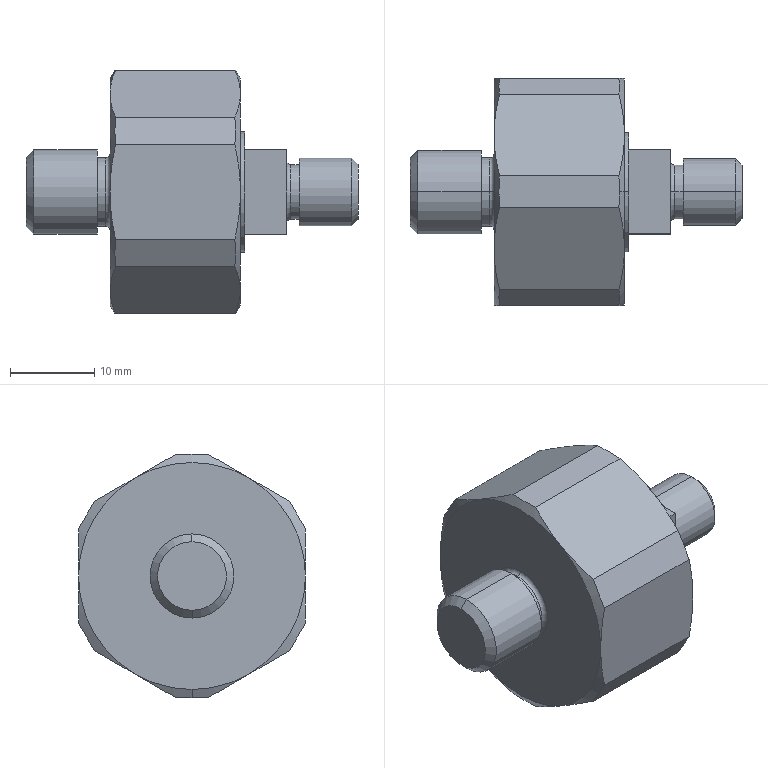Part | STEP file | FJCMXS8-1.25-6 | 1 solid | 56 faces | box 39.5 x 27 x 29 mm | volume 11282 mm3 | plane 24 | cone 18 | cylinder 10 | torus 4 | commonest cylinder face diameters 6.466 x2 8 x2 8.16 x2 10 x2 14.3 x2